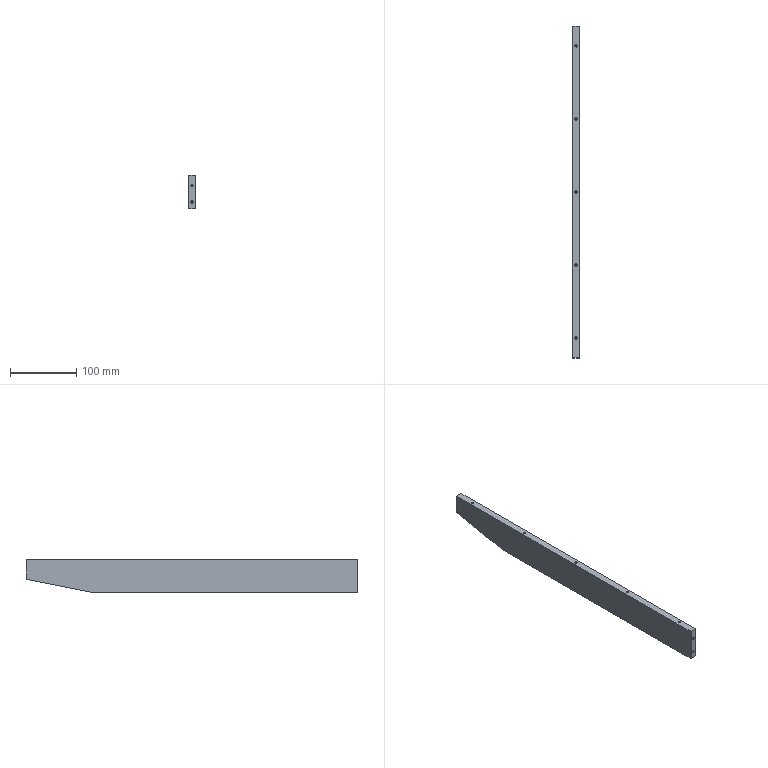Part | STEP file | 03-09 Support plate triangle plate | 1 solid | 35 faces | box 10 x 500 x 50 mm | volume 239136 mm3 | cylinder 14 | cone 14 | plane 7 | commonest cylinder face diameters 3.3 x14